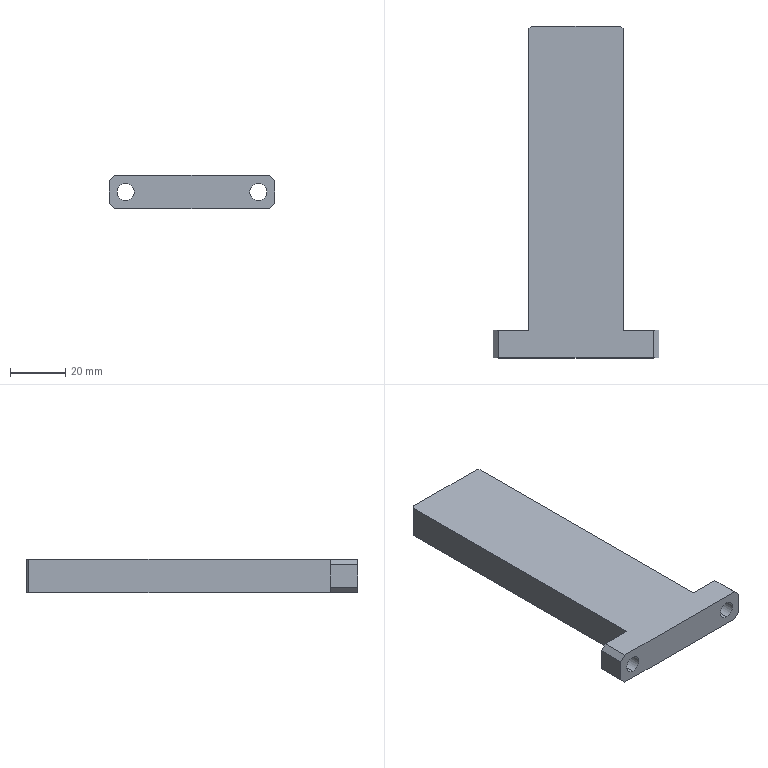Part | STEP file | QA-AD13 | 1 solid | 32 faces | box 60 x 120 x 12 mm | volume 50441 mm3 | plane 16 | cylinder 10 | cone 6 | commonest cylinder face diameters 6 x4 6.2 x4 5 x2